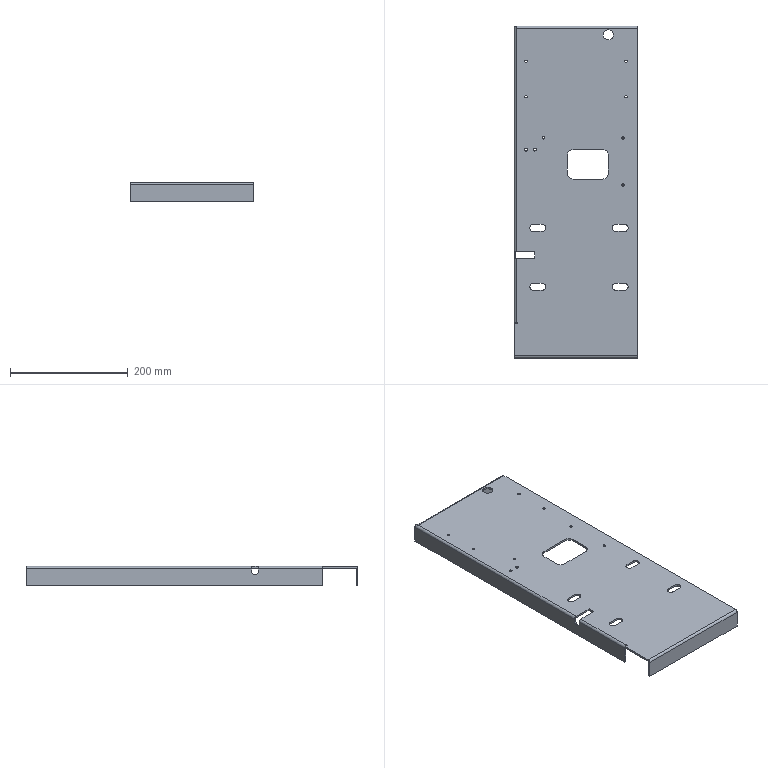Part | STEP file | PN_0081_default | 1 solid | 79 faces | box 210 x 564 x 33 mm | volume 418851 mm3 | plane 48 | cylinder 31 | commonest cylinder face diameters 12 x8 4 x7 2 x4 8 x4 20 x4 5 x2